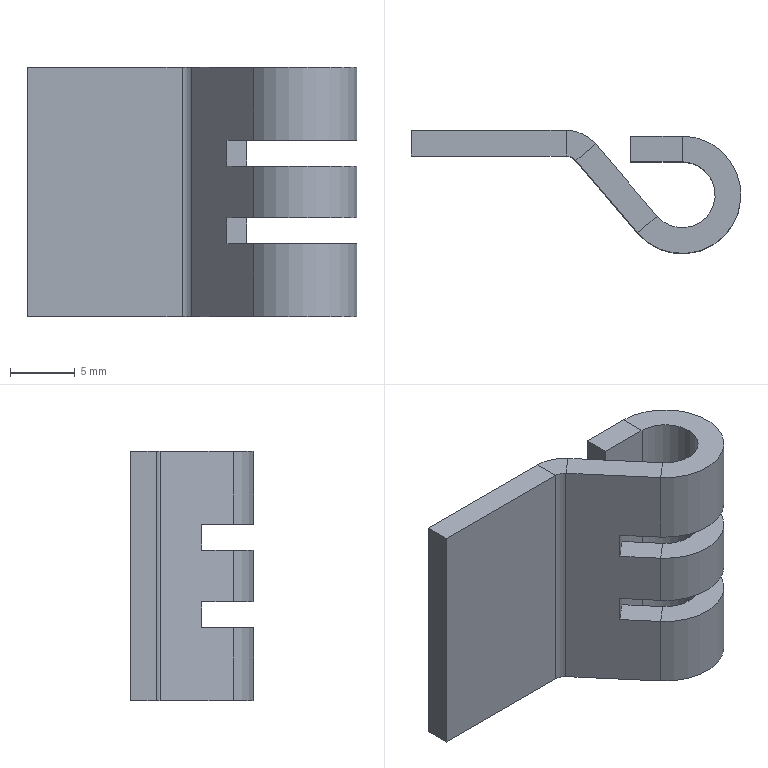Part | SolidWorks | features BaseBody 1 | 1 solid | 46 faces | box 25.55 x 9.55 x 19.3 mm | volume 1346 mm3 | plane 38 | cylinder 8 | commonest cylinder face diameters 5.1 x3 9.1 x3 2 x1 6 x1
STEP:
#1=CARTESIAN_POINT('',(15.,-2.45,-4.));
#2=VERTEX_POINT('',#1);
#3=CARTESIAN_POINT('',(15.,-0.45,-4.));
#4=VERTEX_POINT('',#3);
#5=CARTESIAN_POINT('',(15.,-2.45,-4.));
#6=DIRECTION('',(0.,1.,0.));
#7=VECTOR('',#6,1000.);
#8=LINE('',#5,#7);
#9=EDGE_CURVE('',#2,#4,#8,.T.);
#10=ORIENTED_EDGE('',*,*,#9,.F.);
#11=CARTESIAN_POINT('',(13.06,-6.655,-4.));
#12=VERTEX_POINT('',#11);
#13=CARTESIAN_POINT('',(15.,-5.,-4.));
#14=DIRECTION('',(0.,0.,1.));
#15=DIRECTION('',(-1.,0.,0.));
#16=AXIS2_PLACEMENT_3D('',#13,#14,#15);
#17=CIRCLE('',#16,2.55);
#18=EDGE_CURVE('',#12,#2,#17,.T.);
#19=ORIENTED_EDGE('',*,*,#18,.F.);
#20=CARTESIAN_POINT('',(11.538,-7.953,-4.));
#21=VERTEX_POINT('',#20);
#22=CARTESIAN_POINT('',(11.538,-7.953,-4.));
#23=DIRECTION('',(0.7609,0.6489,0.));
#24=VECTOR('',#23,1000.);
#25=LINE('',#22,#24);
#26=EDGE_CURVE('',#21,#12,#25,.T.);
#27=ORIENTED_EDGE('',*,*,#26,.F.);
#28=CARTESIAN_POINT('',(15.,-5.,-4.));
#29=DIRECTION('',(0.,0.,1.));
#30=DIRECTION('',(-1.,0.,0.));
#31=AXIS2_PLACEMENT_3D('',#28,#29,#30);
#32=CIRCLE('',#31,4.55);
#33=EDGE_CURVE('',#21,#4,#32,.T.);
#34=ORIENTED_EDGE('',*,*,#33,.T.);
#35=EDGE_LOOP('',(#10,#19,#27,#34));
#36=FACE_OUTER_BOUND('',#35,.T.);
#37=CARTESIAN_POINT('',(15.,-5.,-4.));
#38=DIRECTION('',(0.,0.,1.));
#39=DIRECTION('',(1.,0.,0.));
#40=AXIS2_PLACEMENT_3D('',#37,#38,#39);
#41=PLANE('',#40);
#42=ADVANCED_FACE('',(#36),#41,.T.);
#43=CARTESIAN_POINT('',(11.538,-7.953,-2.));
#44=VERTEX_POINT('',#43);
#45=CARTESIAN_POINT('',(13.06,-6.655,-2.));
#46=VERTEX_POINT('',#45);
#47=CARTESIAN_POINT('',(11.538,-7.953,-2.));
#48=DIRECTION('',(0.7609,0.6489,0.));
#49=VECTOR('',#48,1000.);
#50=LINE('',#47,#49);
#51=EDGE_CURVE('',#44,#46,#50,.T.);
#52=ORIENTED_EDGE('',*,*,#51,.T.);
#53=CARTESIAN_POINT('',(15.,-2.45,-2.));
#54=VERTEX_POINT('',#53);
#55=CARTESIAN_POINT('',(15.,-5.,-2.));
#56=DIRECTION('',(0.,0.,-1.));
#57=DIRECTION('',(1.,0.,0.));
#58=AXIS2_PLACEMENT_3D('',#55,#56,#57);
#59=CIRCLE('',#58,2.55);
#60=EDGE_CURVE('',#54,#46,#59,.T.);
#61=ORIENTED_EDGE('',*,*,#60,.F.);
#62=CARTESIAN_POINT('',(15.,-0.45,-2.));
#63=VERTEX_POINT('',#62);
#64=CARTESIAN_POINT('',(15.,-2.45,-2.));
#65=DIRECTION('',(0.,1.,0.));
#66=VECTOR('',#65,1000.);
#67=LINE('',#64,#66);
#68=EDGE_CURVE('',#54,#63,#67,.T.);
#69=ORIENTED_EDGE('',*,*,#68,.T.);
#70=CARTESIAN_POINT('',(15.,-5.,-2.));
#71=DIRECTION('',(0.,0.,-1.));
#72=DIRECTION('',(-1.,0.,0.));
#73=AXIS2_PLACEMENT_3D('',#70,#71,#72);
#74=CIRCLE('',#73,4.55);
#75=EDGE_CURVE('',#63,#44,#74,.T.);
#76=ORIENTED_EDGE('',*,*,#75,.T.);
#77=EDGE_LOOP('',(#52,#61,#69,#76));
#78=FACE_OUTER_BOUND('',#77,.T.);
#79=CARTESIAN_POINT('',(15.,-5.,-2.));
#80=DIRECTION('',(0.,0.,-1.));
#81=DIRECTION('',(0.,-1.,0.));
#82=AXIS2_PLACEMENT_3D('',#79,#80,#81);
#83=PLANE('',#82);
#84=ADVANCED_FACE('',(#78),#83,.T.);
#85=CARTESIAN_POINT('',(11.,-2.45,-4.));
#86=VERTEX_POINT('',#85);
#87=CARTESIAN_POINT('',(11.,-0.45,-4.));
#88=VERTEX_POINT('',#87);
#89=CARTESIAN_POINT('',(11.,-2.45,-4.));
#90=DIRECTION('',(0.,1.,0.));
#91=VECTOR('',#90,1000.);
#92=LINE('',#89,#91);
#93=EDGE_CURVE('',#86,#88,#92,.T.);
#94=ORIENTED_EDGE('',*,*,#93,.F.);
#95=CARTESIAN_POINT('',(15.,-2.45,-4.));
#96=DIRECTION('',(-1.,0.,0.));
#97=VECTOR('',#96,1000.);
#98=LINE('',#95,#97);
#99=EDGE_CURVE('',#2,#86,#98,.T.);
#100=ORIENTED_EDGE('',*,*,#99,.F.);
#101=ORIENTED_EDGE('',*,*,#9,.T.);
#102=CARTESIAN_POINT('',(15.,-0.45,-4.));
#103=DIRECTION('',(-1.,0.,0.));
#104=VECTOR('',#103,1000.);
#105=LINE('',#102,#104);
#106=EDGE_CURVE('',#4,#88,#105,.T.);
#107=ORIENTED_EDGE('',*,*,#106,.T.);
#108=EDGE_LOOP('',(#94,#100,#101,#107));
#109=FACE_OUTER_BOUND('',#108,.T.);
#110=CARTESIAN_POINT('',(15.,-2.45,-4.));
#111=DIRECTION('',(0.,0.,-1.));
#112=DIRECTION('',(0.,-1.,0.));
#113=AXIS2_PLACEMENT_3D('',#110,#111,#112);
#114=PLANE('',#113);
#115=ADVANCED_FACE('',(#109),#114,.F.);
#116=ORIENTED_EDGE('',*,*,#68,.F.);
#117=CARTESIAN_POINT('',(11.,-2.45,-2.));
#118=VERTEX_POINT('',#117);
#119=CARTESIAN_POINT('',(15.,-2.45,-2.));
#120=DIRECTION('',(1.,0.,0.));
#121=VECTOR('',#120,1000.);
#122=LINE('',#119,#121);
#123=EDGE_CURVE('',#118,#54,#122,.T.);
#124=ORIENTED_EDGE('',*,*,#123,.F.);
#125=CARTESIAN_POINT('',(11.,-0.45,-2.));
#126=VERTEX_POINT('',#125);
#127=CARTESIAN_POINT('',(11.,-2.45,-2.));
#128=DIRECTION('',(0.,1.,0.));
#129=VECTOR('',#128,1000.);
#130=LINE('',#127,#129);
#131=EDGE_CURVE('',#118,#126,#130,.T.);
#132=ORIENTED_EDGE('',*,*,#131,.T.);
#133=CARTESIAN_POINT('',(15.,-0.45,-2.));
#134=DIRECTION('',(1.,0.,0.));
#135=VECTOR('',#134,1000.);
#136=LINE('',#133,#135);
#137=EDGE_CURVE('',#126,#63,#136,.T.);
#138=ORIENTED_EDGE('',*,*,#137,.T.);
#139=EDGE_LOOP('',(#116,#124,#132,#138));
#140=FACE_OUTER_BOUND('',#139,.T.);
#141=CARTESIAN_POINT('',(15.,-2.45,-2.));
#142=DIRECTION('',(0.,0.,1.));
#143=DIRECTION('',(1.,0.,0.));
#144=AXIS2_PLACEMENT_3D('',#141,#142,#143);
#145=PLANE('',#144);
#146=ADVANCED_FACE('',(#140),#145,.F.);
#147=CARTESIAN_POINT('',(11.,-4.24,-2.));
#148=VERTEX_POINT('',#147);
#149=CARTESIAN_POINT('',(11.,-4.24,-4.));
#150=VERTEX_POINT('',#149);
#151=CARTESIAN_POINT('',(11.,-4.24,9.65));
#152=DIRECTION('',(0.,0.,-1.));
#153=VECTOR('',#152,1000.);
#154=LINE('',#151,#153);
#155=EDGE_CURVE('',#148,#150,#154,.T.);
#156=ORIENTED_EDGE('',*,*,#155,.F.);
#157=CARTESIAN_POINT('',(9.478,-5.537,-2.));
#158=VERTEX_POINT('',#157);
#159=CARTESIAN_POINT('',(11.,-4.24,-2.));
#160=DIRECTION('',(-0.7609,-0.6489,0.));
#161=VECTOR('',#160,1000.);
#162=LINE('',#159,#161);
#163=EDGE_CURVE('',#148,#158,#162,.T.);
#164=ORIENTED_EDGE('',*,*,#163,.T.);
#165=CARTESIAN_POINT('',(9.478,-5.537,-4.));
#166=VERTEX_POINT('',#165);
#167=CARTESIAN_POINT('',(9.478,-5.537,9.65));
#168=DIRECTION('',(0.,0.,-1.));
#169=VECTOR('',#168,1000.);
#170=LINE('',#167,#169);
#171=EDGE_CURVE('',#158,#166,#170,.T.);
#172=ORIENTED_EDGE('',*,*,#171,.T.);
#173=CARTESIAN_POINT('',(11.,-4.24,-4.));
#174=DIRECTION('',(-0.7609,-0.6489,0.));
#175=VECTOR('',#174,1000.);
#176=LINE('',#173,#175);
#177=EDGE_CURVE('',#150,#166,#176,.T.);
#178=ORIENTED_EDGE('',*,*,#177,.F.);
#179=EDGE_LOOP('',(#156,#164,#172,#178));
#180=FACE_OUTER_BOUND('',#179,.T.);
#181=CARTESIAN_POINT('',(11.,-4.24,9.65));
#182=DIRECTION('',(-0.6489,0.7609,0.));
#183=DIRECTION('',(0.,0.,1.));
#184=AXIS2_PLACEMENT_3D('',#181,#182,#183);
#185=PLANE('',#184);
#186=ADVANCED_FACE('',(#180),#185,.F.);
#187=CARTESIAN_POINT('',(11.538,-7.953,-4.));
#188=DIRECTION('',(0.6489,-0.7609,0.));
#189=VECTOR('',#188,1000.);
#190=LINE('',#187,#189);
#191=EDGE_CURVE('',#166,#21,#190,.T.);
#192=ORIENTED_EDGE('',*,*,#191,.T.);
#193=ORIENTED_EDGE('',*,*,#26,.T.);
#194=CARTESIAN_POINT('',(13.06,-6.655,-4.));
#195=DIRECTION('',(0.6489,-0.7609,0.));
#196=VECTOR('',#195,1000.);
#197=LINE('',#194,#196);
#198=EDGE_CURVE('',#150,#12,#197,.T.);
#199=ORIENTED_EDGE('',*,*,#198,.F.);
#200=ORIENTED_EDGE('',*,*,#177,.T.);
#201=EDGE_LOOP('',(#192,#193,#199,#200));
#202=FACE_OUTER_BOUND('',#201,.T.);
#203=CARTESIAN_POINT('',(11.538,-7.953,-4.));
#204=DIRECTION('',(0.,0.,-1.));
#205=DIRECTION('',(0.,-1.,0.));
#206=AXIS2_PLACEMENT_3D('',#203,#204,#205);
#207=PLANE('',#206);
#208=ADVANCED_FACE('',(#202),#207,.F.);
#209=ORIENTED_EDGE('',*,*,#51,.F.);
#210=CARTESIAN_POINT('',(11.538,-7.953,-2.));
#211=DIRECTION('',(-0.6489,0.7609,0.));
#212=VECTOR('',#211,1000.);
#213=LINE('',#210,#212);
#214=EDGE_CURVE('',#44,#158,#213,.T.);
#215=ORIENTED_EDGE('',*,*,#214,.T.);
#216=ORIENTED_EDGE('',*,*,#163,.F.);
#217=CARTESIAN_POINT('',(13.06,-6.655,-2.));
#218=DIRECTION('',(-0.6489,0.7609,0.));
#219=VECTOR('',#218,1000.);
#220=LINE('',#217,#219);
#221=EDGE_CURVE('',#46,#148,#220,.T.);
#222=ORIENTED_EDGE('',*,*,#221,.F.);
#223=EDGE_LOOP('',(#209,#215,#216,#222));
#224=FACE_OUTER_BOUND('',#223,.T.);
#225=CARTESIAN_POINT('',(11.538,-7.953,-2.));
#226=DIRECTION('',(0.,0.,1.));
#227=DIRECTION('',(0.,-1.,0.));
#228=AXIS2_PLACEMENT_3D('',#225,#226,#227);
#229=PLANE('',#228);
#230=ADVANCED_FACE('',(#224),#229,.F.);
#231=CARTESIAN_POINT('',(11.538,-7.953,4.));
#232=VERTEX_POINT('',#231);
#233=CARTESIAN_POINT('',(13.06,-6.655,4.));
#234=VERTEX_POINT('',#233);
#235=CARTESIAN_POINT('',(11.538,-7.953,4.));
#236=DIRECTION('',(0.7609,0.6489,0.));
#237=VECTOR('',#236,1000.);
#238=LINE('',#235,#237);
#239=EDGE_CURVE('',#232,#234,#238,.T.);
#240=ORIENTED_EDGE('',*,*,#239,.T.);
#241=CARTESIAN_POINT('',(15.,-2.45,4.));
#242=VERTEX_POINT('',#241);
#243=CARTESIAN_POINT('',(15.,-5.,4.));
#244=DIRECTION('',(0.,0.,-1.));
#245=DIRECTION('',(1.,0.,0.));
#246=AXIS2_PLACEMENT_3D('',#243,#244,#245);
#247=CIRCLE('',#246,2.55);
#248=EDGE_CURVE('',#242,#234,#247,.T.);
#249=ORIENTED_EDGE('',*,*,#248,.F.);
#250=CARTESIAN_POINT('',(15.,-0.45,4.));
#251=VERTEX_POINT('',#250);
#252=CARTESIAN_POINT('',(15.,-2.45,4.));
#253=DIRECTION('',(0.,1.,0.));
#254=VECTOR('',#253,1000.);
#255=LINE('',#252,#254);
#256=EDGE_CURVE('',#242,#251,#255,.T.);
#257=ORIENTED_EDGE('',*,*,#256,.T.);
#258=CARTESIAN_POINT('',(15.,-5.,4.));
#259=DIRECTION('',(0.,0.,-1.));
#260=DIRECTION('',(-1.,0.,0.));
#261=AXIS2_PLACEMENT_3D('',#258,#259,#260);
#262=CIRCLE('',#261,4.55);
#263=EDGE_CURVE('',#251,#232,#262,.T.);
#264=ORIENTED_EDGE('',*,*,#263,.T.);
#265=EDGE_LOOP('',(#240,#249,#257,#264));
#266=FACE_OUTER_BOUND('',#265,.T.);
#267=CARTESIAN_POINT('',(15.,-5.,4.));
#268=DIRECTION('',(0.,0.,-1.));
#269=DIRECTION('',(0.,-1.,0.));
#270=AXIS2_PLACEMENT_3D('',#267,#268,#269);
#271=PLANE('',#270);
#272=ADVANCED_FACE('',(#266),#271,.T.);
#273=CARTESIAN_POINT('',(15.,-2.45,2.));
#274=VERTEX_POINT('',#273);
#275=CARTESIAN_POINT('',(15.,-0.45,2.));
#276=VERTEX_POINT('',#275);
#277=CARTESIAN_POINT('',(15.,-2.45,2.));
#278=DIRECTION('',(0.,1.,0.));
#279=VECTOR('',#278,1000.);
#280=LINE('',#277,#279);
#281=EDGE_CURVE('',#274,#276,#280,.T.);
#282=ORIENTED_EDGE('',*,*,#281,.F.);
#283=CARTESIAN_POINT('',(13.06,-6.655,2.));
#284=VERTEX_POINT('',#283);
#285=CARTESIAN_POINT('',(15.,-5.,2.));
#286=DIRECTION('',(0.,0.,1.));
#287=DIRECTION('',(-1.,0.,0.));
#288=AXIS2_PLACEMENT_3D('',#285,#286,#287);
#289=CIRCLE('',#288,2.55);
#290=EDGE_CURVE('',#284,#274,#289,.T.);
#291=ORIENTED_EDGE('',*,*,#290,.F.);
#292=CARTESIAN_POINT('',(11.538,-7.953,2.));
#293=VERTEX_POINT('',#292);
#294=CARTESIAN_POINT('',(11.538,-7.953,2.));
#295=DIRECTION('',(0.7609,0.6489,0.));
#296=VECTOR('',#295,1000.);
#297=LINE('',#294,#296);
#298=EDGE_CURVE('',#293,#284,#297,.T.);
#299=ORIENTED_EDGE('',*,*,#298,.F.);
#300=CARTESIAN_POINT('',(15.,-5.,2.));
#301=DIRECTION('',(0.,0.,1.));
#302=DIRECTION('',(-1.,0.,0.));
#303=AXIS2_PLACEMENT_3D('',#300,#301,#302);
#304=CIRCLE('',#303,4.55);
#305=EDGE_CURVE('',#293,#276,#304,.T.);
#306=ORIENTED_EDGE('',*,*,#305,.T.);
#307=EDGE_LOOP('',(#282,#291,#299,#306));
#308=FACE_OUTER_BOUND('',#307,.T.);
#309=CARTESIAN_POINT('',(15.,-5.,2.));
#310=DIRECTION('',(0.,0.,1.));
#311=DIRECTION('',(1.,0.,0.));
#312=AXIS2_PLACEMENT_3D('',#309,#310,#311);
#313=PLANE('',#312);
#314=ADVANCED_FACE('',(#308),#313,.T.);
#315=ORIENTED_EDGE('',*,*,#256,.F.);
#316=CARTESIAN_POINT('',(11.,-2.45,4.));
#317=VERTEX_POINT('',#316);
#318=CARTESIAN_POINT('',(15.,-2.45,4.));
#319=DIRECTION('',(1.,0.,0.));
#320=VECTOR('',#319,1000.);
#321=LINE('',#318,#320);
#322=EDGE_CURVE('',#317,#242,#321,.T.);
#323=ORIENTED_EDGE('',*,*,#322,.F.);
#324=CARTESIAN_POINT('',(11.,-0.45,4.));
#325=VERTEX_POINT('',#324);
#326=CARTESIAN_POINT('',(11.,-2.45,4.));
#327=DIRECTION('',(0.,1.,0.));
#328=VECTOR('',#327,1000.);
#329=LINE('',#326,#328);
#330=EDGE_CURVE('',#317,#325,#329,.T.);
#331=ORIENTED_EDGE('',*,*,#330,.T.);
#332=CARTESIAN_POINT('',(15.,-0.45,4.));
#333=DIRECTION('',(1.,0.,0.));
#334=VECTOR('',#333,1000.);
#335=LINE('',#332,#334);
#336=EDGE_CURVE('',#325,#251,#335,.T.);
#337=ORIENTED_EDGE('',*,*,#336,.T.);
#338=EDGE_LOOP('',(#315,#323,#331,#337));
#339=FACE_OUTER_BOUND('',#338,.T.);
#340=CARTESIAN_POINT('',(15.,-2.45,4.));
#341=DIRECTION('',(0.,0.,1.));
#342=DIRECTION('',(1.,0.,0.));
#343=AXIS2_PLACEMENT_3D('',#340,#341,#342);
#344=PLANE('',#343);
#345=ADVANCED_FACE('',(#339),#344,.F.);
#346=CARTESIAN_POINT('',(11.,-2.45,2.));
#347=VERTEX_POINT('',#346);
#348=CARTESIAN_POINT('',(11.,-0.45,2.));
#349=VERTEX_POINT('',#348);
#350=CARTESIAN_POINT('',(11.,-2.45,2.));
#351=DIRECTION('',(0.,1.,0.));
#352=VECTOR('',#351,1000.);
#353=LINE('',#350,#352);
#354=EDGE_CURVE('',#347,#349,#353,.T.);
#355=ORIENTED_EDGE('',*,*,#354,.F.);
#356=CARTESIAN_POINT('',(15.,-2.45,2.));
#357=DIRECTION('',(-1.,0.,0.));
#358=VECTOR('',#357,1000.);
#359=LINE('',#356,#358);
#360=EDGE_CURVE('',#274,#347,#359,.T.);
#361=ORIENTED_EDGE('',*,*,#360,.F.);
#362=ORIENTED_EDGE('',*,*,#281,.T.);
#363=CARTESIAN_POINT('',(15.,-0.45,2.));
#364=DIRECTION('',(-1.,0.,0.));
#365=VECTOR('',#364,1000.);
#366=LINE('',#363,#365);
#367=EDGE_CURVE('',#276,#349,#366,.T.);
#368=ORIENTED_EDGE('',*,*,#367,.T.);
#369=EDGE_LOOP('',(#355,#361,#362,#368));
#370=FACE_OUTER_BOUND('',#369,.T.);
#371=CARTESIAN_POINT('',(15.,-2.45,2.));
#372=DIRECTION('',(0.,0.,-1.));
#373=DIRECTION('',(-1.,0.,0.));
#374=AXIS2_PLACEMENT_3D('',#371,#372,#373);
#375=PLANE('',#374);
#376=ADVANCED_FACE('',(#370),#375,.F.);
#377=CARTESIAN_POINT('',(11.,-4.24,2.));
#378=VERTEX_POINT('',#377);
#379=CARTESIAN_POINT('',(9.478,-5.537,2.));
#380=VERTEX_POINT('',#379);
#381=CARTESIAN_POINT('',(11.,-4.24,2.));
#382=DIRECTION('',(-0.7609,-0.6489,0.));
#383=VECTOR('',#382,1000.);
#384=LINE('',#381,#383);
#385=EDGE_CURVE('',#378,#380,#384,.T.);
#386=ORIENTED_EDGE('',*,*,#385,.F.);
#387=CARTESIAN_POINT('',(11.,-4.24,4.));
#388=VERTEX_POINT('',#387);
#389=CARTESIAN_POINT('',(11.,-4.24,9.65));
#390=DIRECTION('',(0.,0.,-1.));
#391=VECTOR('',#390,1000.);
#392=LINE('',#389,#391);
#393=EDGE_CURVE('',#388,#378,#392,.T.);
#394=ORIENTED_EDGE('',*,*,#393,.F.);
#395=CARTESIAN_POINT('',(9.478,-5.537,4.));
#396=VERTEX_POINT('',#395);
#397=CARTESIAN_POINT('',(11.,-4.24,4.));
#398=DIRECTION('',(-0.7609,-0.6489,0.));
#399=VECTOR('',#398,1000.);
#400=LINE('',#397,#399);
#401=EDGE_CURVE('',#388,#396,#400,.T.);
#402=ORIENTED_EDGE('',*,*,#401,.T.);
#403=CARTESIAN_POINT('',(9.478,-5.537,9.65));
#404=DIRECTION('',(0.,0.,-1.));
#405=VECTOR('',#404,1000.);
#406=LINE('',#403,#405);
#407=EDGE_CURVE('',#396,#380,#406,.T.);
#408=ORIENTED_EDGE('',*,*,#407,.T.);
#409=EDGE_LOOP('',(#386,#394,#402,#408));
#410=FACE_OUTER_BOUND('',#409,.T.);
#411=CARTESIAN_POINT('',(11.,-4.24,9.65));
#412=DIRECTION('',(-0.6489,0.7609,0.));
#413=DIRECTION('',(0.,0.,1.));
#414=AXIS2_PLACEMENT_3D('',#411,#412,#413);
#415=PLANE('',#414);
#416=ADVANCED_FACE('',(#410),#415,.F.);
#417=CARTESIAN_POINT('',(11.538,-7.953,4.));
#418=DIRECTION('',(-0.6489,0.7609,0.));
#419=VECTOR('',#418,1000.);
#420=LINE('',#417,#419);
#421=EDGE_CURVE('',#232,#396,#420,.T.);
#422=ORIENTED_EDGE('',*,*,#421,.T.);
#423=ORIENTED_EDGE('',*,*,#401,.F.);
#424=CARTESIAN_POINT('',(13.06,-6.655,4.));
#425=DIRECTION('',(-0.6489,0.7609,0.));
#426=VECTOR('',#425,1000.);
#427=LINE('',#424,#426);
#428=EDGE_CURVE('',#234,#388,#427,.T.);
#429=ORIENTED_EDGE('',*,*,#428,.F.);
#430=ORIENTED_EDGE('',*,*,#239,.F.);
#431=EDGE_LOOP('',(#422,#423,#429,#430));
#432=FACE_OUTER_BOUND('',#431,.T.);
#433=CARTESIAN_POINT('',(11.538,-7.953,4.));
#434=DIRECTION('',(0.,0.,1.));
#435=DIRECTION('',(1.,0.,0.));
#436=AXIS2_PLACEMENT_3D('',#433,#434,#435);
#437=PLANE('',#436);
#438=ADVANCED_FACE('',(#432),#437,.F.);
#439=CARTESIAN_POINT('',(11.538,-7.953,2.));
#440=DIRECTION('',(0.6489,-0.7609,0.));
#441=VECTOR('',#440,1000.);
#442=LINE('',#439,#441);
#443=EDGE_CURVE('',#380,#293,#442,.T.);
#444=ORIENTED_EDGE('',*,*,#443,.T.);
#445=ORIENTED_EDGE('',*,*,#298,.T.);
#446=CARTESIAN_POINT('',(13.06,-6.655,2.));
#447=DIRECTION('',(0.6489,-0.7609,0.));
#448=VECTOR('',#447,1000.);
#449=LINE('',#446,#448);
#450=EDGE_CURVE('',#378,#284,#449,.T.);
#451=ORIENTED_EDGE('',*,*,#450,.F.);
#452=ORIENTED_EDGE('',*,*,#385,.T.);
#453=EDGE_LOOP('',(#444,#445,#451,#452));
#454=FACE_OUTER_BOUND('',#453,.T.);
#455=CARTESIAN_POINT('',(11.538,-7.953,2.));
#456=DIRECTION('',(0.,0.,-1.));
#457=DIRECTION('',(-1.,0.,0.));
#458=AXIS2_PLACEMENT_3D('',#455,#456,#457);
#459=PLANE('',#458);
#460=ADVANCED_FACE('',(#454),#459,.F.);
#461=CARTESIAN_POINT('',(11.,-0.45,-9.65));
#462=VERTEX_POINT('',#461);
#463=CARTESIAN_POINT('',(15.,-0.45,-9.65));
#464=VERTEX_POINT('',#463);
#465=CARTESIAN_POINT('',(15.,-0.45,-9.65));
#466=DIRECTION('',(1.,0.,0.));
#467=VECTOR('',#466,1000.);
#468=LINE('',#465,#467);
#469=EDGE_CURVE('',#462,#464,#468,.T.);
#470=ORIENTED_EDGE('',*,*,#469,.T.);
#471=CARTESIAN_POINT('',(15.,-2.45,-9.65));
#472=VERTEX_POINT('',#471);
#473=CARTESIAN_POINT('',(15.,-0.45,-9.65));
#474=DIRECTION('',(0.,-1.,0.));
#475=VECTOR('',#474,1000.);
#476=LINE('',#473,#475);
#477=EDGE_CURVE('',#464,#472,#476,.T.);
#478=ORIENTED_EDGE('',*,*,#477,.T.);
#479=CARTESIAN_POINT('',(11.,-2.45,-9.65));
#480=VERTEX_POINT('',#479);
#481=CARTESIAN_POINT('',(15.,-2.45,-9.65));
#482=DIRECTION('',(1.,0.,0.));
#483=VECTOR('',#482,1000.);
#484=LINE('',#481,#483);
#485=EDGE_CURVE('',#480,#472,#484,.T.);
#486=ORIENTED_EDGE('',*,*,#485,.F.);
#487=CARTESIAN_POINT('',(11.,-2.45,-9.65));
#488=DIRECTION('',(0.,1.,0.));
#489=VECTOR('',#488,1000.);
#490=LINE('',#487,#489);
#491=EDGE_CURVE('',#480,#462,#490,.T.);
#492=ORIENTED_EDGE('',*,*,#491,.T.);
#493=EDGE_LOOP('',(#470,#478,#486,#492));
#494=FACE_OUTER_BOUND('',#493,.T.);
#495=CARTESIAN_POINT('',(6.,-3.,-9.65));
#496=DIRECTION('',(0.,0.,1.));
#497=DIRECTION('',(1.,0.,0.));
#498=AXIS2_PLACEMENT_3D('',#495,#496,#497);
#499=PLANE('',#498);
#500=ADVANCED_FACE('',(#494),#499,.F.);
#501=CARTESIAN_POINT('',(6.,0.,9.65));
#502=VERTEX_POINT('',#501);
#503=CARTESIAN_POINT('',(-6.,0.,9.65));
#504=VERTEX_POINT('',#503);
#505=CARTESIAN_POINT('',(6.,0.,9.65));
#506=DIRECTION('',(-1.,0.,0.));
#507=VECTOR('',#506,1000.);
#508=LINE('',#505,#507);
#509=EDGE_CURVE('',#502,#504,#508,.T.);
#510=ORIENTED_EDGE('',*,*,#509,.T.);
#511=CARTESIAN_POINT('',(-6.,-2.,9.65));
#512=VERTEX_POINT('',#511);
#513=CARTESIAN_POINT('',(-6.,-2.,9.65));
#514=DIRECTION('',(0.,1.,0.));
#515=VECTOR('',#514,1000.);
#516=LINE('',#513,#515);
#517=EDGE_CURVE('',#512,#504,#516,.T.);
#518=ORIENTED_EDGE('',*,*,#517,.F.);
#519=CARTESIAN_POINT('',(6.,-2.,9.65));
#520=VERTEX_POINT('',#519);
#521=CARTESIAN_POINT('',(6.,-2.,9.65));
#522=DIRECTION('',(-1.,0.,0.));
#523=VECTOR('',#522,1000.);
#524=LINE('',#521,#523);
#525=EDGE_CURVE('',#520,#512,#524,.T.);
#526=ORIENTED_EDGE('',*,*,#525,.F.);
#527=CARTESIAN_POINT('',(6.,-2.,9.65));
#528=DIRECTION('',(0.,1.,0.));
#529=VECTOR('',#528,1000.);
#530=LINE('',#527,#529);
#531=EDGE_CURVE('',#520,#502,#530,.T.);
#532=ORIENTED_EDGE('',*,*,#531,.T.);
#533=EDGE_LOOP('',(#510,#518,#526,#532));
#534=FACE_OUTER_BOUND('',#533,.T.);
#535=CARTESIAN_POINT('',(6.,-3.,9.65));
#536=DIRECTION('',(0.,0.,1.));
#537=DIRECTION('',(1.,0.,0.));
#538=AXIS2_PLACEMENT_3D('',#535,#536,#537);
#539=PLANE('',#538);
#540=ADVANCED_FACE('',(#534),#539,.T.);
#541=CARTESIAN_POINT('',(8.283,-1.053,-9.65));
#542=VERTEX_POINT('',#541);
#543=CARTESIAN_POINT('',(6.,0.,-9.65));
#544=VERTEX_POINT('',#543);
#545=CARTESIAN_POINT('',(6.,-3.,-9.65));
#546=DIRECTION('',(0.,0.,1.));
#547=DIRECTION('',(1.,0.,0.));
#548=AXIS2_PLACEMENT_3D('',#545,#546,#547);
#549=CIRCLE('',#548,3.);
#550=EDGE_CURVE('',#542,#544,#549,.T.);
#551=ORIENTED_EDGE('',*,*,#550,.T.);
#552=CARTESIAN_POINT('',(6.,0.,9.65));
#553=DIRECTION('',(0.,0.,-1.));
#554=VECTOR('',#553,1000.);
#555=LINE('',#552,#554);
#556=EDGE_CURVE('',#502,#544,#555,.T.);
#557=ORIENTED_EDGE('',*,*,#556,.F.);
#558=CARTESIAN_POINT('',(8.283,-1.053,9.65));
#559=VERTEX_POINT('',#558);
#560=CARTESIAN_POINT('',(6.,-3.,9.65));
#561=DIRECTION('',(0.,0.,1.));
#562=DIRECTION('',(1.,0.,0.));
#563=AXIS2_PLACEMENT_3D('',#560,#561,#562);
#564=CIRCLE('',#563,3.);
#565=EDGE_CURVE('',#559,#502,#564,.T.);
#566=ORIENTED_EDGE('',*,*,#565,.F.);
#567=CARTESIAN_POINT('',(8.283,-1.053,9.65));
#568=DIRECTION('',(0.,0.,-1.));
#569=VECTOR('',#568,1000.);
#570=LINE('',#567,#569);
#571=EDGE_CURVE('',#559,#542,#570,.T.);
#572=ORIENTED_EDGE('',*,*,#571,.T.);
#573=EDGE_LOOP('',(#551,#557,#566,#572));
#574=FACE_OUTER_BOUND('',#573,.T.);
#575=CARTESIAN_POINT('',(6.,-3.,9.65));
#576=DIRECTION('',(0.,0.,-1.));
#577=DIRECTION('',(-1.,0.,0.));
#578=AXIS2_PLACEMENT_3D('',#575,#576,#577);
#579=CYLINDRICAL_SURFACE('',#578,3.);
#580=ADVANCED_FACE('',(#574),#579,.T.);
#581=CARTESIAN_POINT('',(6.761,-2.351,-9.65));
#582=VERTEX_POINT('',#581);
#583=CARTESIAN_POINT('',(6.,-2.,-9.65));
#584=VERTEX_POINT('',#583);
#585=CARTESIAN_POINT('',(6.,-3.,-9.65));
#586=DIRECTION('',(0.,0.,1.));
#587=DIRECTION('',(1.,0.,0.));
#588=AXIS2_PLACEMENT_3D('',#585,#586,#587);
#589=CIRCLE('',#588,1.);
#590=EDGE_CURVE('',#582,#584,#589,.T.);
#591=ORIENTED_EDGE('',*,*,#590,.F.);
#592=CARTESIAN_POINT('',(6.761,-2.351,9.65));
#593=VERTEX_POINT('',#592);
#594=CARTESIAN_POINT('',(6.761,-2.351,9.65));
#595=DIRECTION('',(0.,0.,-1.));
#596=VECTOR('',#595,1000.);
#597=LINE('',#594,#596);
#598=EDGE_CURVE('',#593,#582,#597,.T.);
#599=ORIENTED_EDGE('',*,*,#598,.F.);
#600=CARTESIAN_POINT('',(6.,-3.,9.65));
#601=DIRECTION('',(0.,0.,1.));
#602=DIRECTION('',(1.,0.,0.));
#603=AXIS2_PLACEMENT_3D('',#600,#601,#602);
#604=CIRCLE('',#603,1.);
#605=EDGE_CURVE('',#593,#520,#604,.T.);
#606=ORIENTED_EDGE('',*,*,#605,.T.);
#607=CARTESIAN_POINT('',(6.,-2.,9.65));
#608=DIRECTION('',(0.,0.,-1.));
#609=VECTOR('',#608,1000.);
#610=LINE('',#607,#609);
#611=EDGE_CURVE('',#520,#584,#610,.T.);
#612=ORIENTED_EDGE('',*,*,#611,.T.);
#613=EDGE_LOOP('',(#591,#599,#606,#612));
#614=FACE_OUTER_BOUND('',#613,.T.);
#615=CARTESIAN_POINT('',(6.,-3.,9.65));
#616=DIRECTION('',(0.,0.,-1.));
#617=DIRECTION('',(-1.,0.,0.));
#618=AXIS2_PLACEMENT_3D('',#615,#616,#617);
#619=CYLINDRICAL_SURFACE('',#618,1.);
#620=ADVANCED_FACE('',(#614),#619,.F.);
#621=ORIENTED_EDGE('',*,*,#525,.T.);
#622=CARTESIAN_POINT('',(-6.,-2.,-9.65));
#623=VERTEX_POINT('',#622);
#624=CARTESIAN_POINT('',(-6.,-2.,9.65));
#625=DIRECTION('',(0.,0.,-1.));
#626=VECTOR('',#625,1000.);
#627=LINE('',#624,#626);
#628=EDGE_CURVE('',#512,#623,#627,.T.);
#629=ORIENTED_EDGE('',*,*,#628,.T.);
#630=CARTESIAN_POINT('',(6.,-2.,-9.65));
#631=DIRECTION('',(-1.,0.,0.));
#632=VECTOR('',#631,1000.);
#633=LINE('',#630,#632);
#634=EDGE_CURVE('',#584,#623,#633,.T.);
#635=ORIENTED_EDGE('',*,*,#634,.F.);
#636=ORIENTED_EDGE('',*,*,#611,.F.);
#637=EDGE_LOOP('',(#621,#629,#635,#636));
#638=FACE_OUTER_BOUND('',#637,.T.);
#639=CARTESIAN_POINT('',(6.,-2.,9.65));
#640=DIRECTION('',(0.,-1.,0.));
#641=DIRECTION('',(0.,0.,-1.));
#642=AXIS2_PLACEMENT_3D('',#639,#640,#641);
#643=PLANE('',#642);
#644=ADVANCED_FACE('',(#638),#643,.T.);
#645=CARTESIAN_POINT('',(-6.,0.,-9.65));
#646=VERTEX_POINT('',#645);
#647=CARTESIAN_POINT('',(-6.,-2.,-9.65));
#648=DIRECTION('',(0.,1.,0.));
#649=VECTOR('',#648,1000.);
#650=LINE('',#647,#649);
#651=EDGE_CURVE('',#623,#646,#650,.T.);
#652=ORIENTED_EDGE('',*,*,#651,.F.);
#653=ORIENTED_EDGE('',*,*,#628,.F.);
#654=ORIENTED_EDGE('',*,*,#517,.T.);
#655=CARTESIAN_POINT('',(-6.,0.,9.65));
#656=DIRECTION('',(0.,0.,-1.));
#657=VECTOR('',#656,1000.);
#658=LINE('',#655,#657);
#659=EDGE_CURVE('',#504,#646,#658,.T.);
#660=ORIENTED_EDGE('',*,*,#659,.T.);
#661=EDGE_LOOP('',(#652,#653,#654,#660));
#662=FACE_OUTER_BOUND('',#661,.T.);
#663=CARTESIAN_POINT('',(-6.,-2.,9.65));
#664=DIRECTION('',(-1.,0.,0.));
#665=DIRECTION('',(0.,1.,0.));
#666=AXIS2_PLACEMENT_3D('',#663,#664,#665);
#667=PLANE('',#666);
#668=ADVANCED_FACE('',(#662),#667,.T.);
#669=CARTESIAN_POINT('',(6.,0.,-9.65));
#670=DIRECTION('',(-1.,0.,0.));
#671=VECTOR('',#670,1000.);
#672=LINE('',#669,#671);
#673=EDGE_CURVE('',#544,#646,#672,.T.);
#674=ORIENTED_EDGE('',*,*,#673,.T.);
#675=ORIENTED_EDGE('',*,*,#659,.F.);
#676=ORIENTED_EDGE('',*,*,#509,.F.);
#677=ORIENTED_EDGE('',*,*,#556,.T.);
#678=EDGE_LOOP('',(#674,#675,#676,#677));
#679=FACE_OUTER_BOUND('',#678,.T.);
#680=CARTESIAN_POINT('',(6.,0.,9.65));
#681=DIRECTION('',(0.,-1.,0.));
#682=DIRECTION('',(0.,0.,-1.));
#683=AXIS2_PLACEMENT_3D('',#680,#681,#682);
#684=PLANE('',#683);
#685=ADVANCED_FACE('',(#679),#684,.F.);
#686=ORIENTED_EDGE('',*,*,#634,.T.);
#687=ORIENTED_EDGE('',*,*,#651,.T.);
#688=ORIENTED_EDGE('',*,*,#673,.F.);
#689=CARTESIAN_POINT('',(6.,0.,-9.65));
#690=DIRECTION('',(0.,-1.,0.));
#691=VECTOR('',#690,1000.);
#692=LINE('',#689,#691);
#693=EDGE_CURVE('',#544,#584,#692,.T.);
#694=ORIENTED_EDGE('',*,*,#693,.T.);
#695=EDGE_LOOP('',(#686,#687,#688,#694));
#696=FACE_OUTER_BOUND('',#695,.T.);
#697=CARTESIAN_POINT('',(6.761,-2.351,-9.65));
#698=DIRECTION('',(0.,0.,-1.));
#699=DIRECTION('',(0.,-1.,0.));
#700=AXIS2_PLACEMENT_3D('',#697,#698,#699);
#701=PLANE('',#700);
#702=ADVANCED_FACE('',(#696),#701,.T.);
#703=ORIENTED_EDGE('',*,*,#693,.F.);
#704=ORIENTED_EDGE('',*,*,#550,.F.);
#705=CARTESIAN_POINT('',(6.761,-2.351,-9.65));
#706=DIRECTION('',(0.7609,0.6489,0.));
#707=VECTOR('',#706,1000.);
#708=LINE('',#705,#707);
#709=EDGE_CURVE('',#582,#542,#708,.T.);
#710=ORIENTED_EDGE('',*,*,#709,.F.);
#711=ORIENTED_EDGE('',*,*,#590,.T.);
#712=EDGE_LOOP('',(#703,#704,#710,#711));
#713=FACE_OUTER_BOUND('',#712,.T.);
#714=CARTESIAN_POINT('',(6.,0.,-9.65));
#715=DIRECTION('',(0.,0.,-1.));
#716=DIRECTION('',(0.,-1.,0.));
#717=AXIS2_PLACEMENT_3D('',#714,#715,#716);
#718=PLANE('',#717);
#719=ADVANCED_FACE('',(#713),#718,.T.);
#720=CARTESIAN_POINT('',(13.06,-6.655,9.65));
#721=VERTEX_POINT('',#720);
#722=CARTESIAN_POINT('',(13.06,-6.655,9.65));
#723=DIRECTION('',(-0.6489,0.7609,0.));
#724=VECTOR('',#723,1000.);
#725=LINE('',#722,#724);
#726=EDGE_CURVE('',#721,#559,#725,.T.);
#727=ORIENTED_EDGE('',*,*,#726,.T.);
#728=CARTESIAN_POINT('',(8.283,-1.053,9.65));
#729=DIRECTION('',(-0.7609,-0.6489,0.));
#730=VECTOR('',#729,1000.);
#731=LINE('',#728,#730);
#732=EDGE_CURVE('',#559,#593,#731,.T.);
#733=ORIENTED_EDGE('',*,*,#732,.T.);
#734=CARTESIAN_POINT('',(11.538,-7.953,9.65));
#735=VERTEX_POINT('',#734);
#736=CARTESIAN_POINT('',(11.538,-7.953,9.65));
#737=DIRECTION('',(-0.6489,0.7609,0.));
#738=VECTOR('',#737,1000.);
#739=LINE('',#736,#738);
#740=EDGE_CURVE('',#735,#593,#739,.T.);
#741=ORIENTED_EDGE('',*,*,#740,.F.);
#742=CARTESIAN_POINT('',(11.538,-7.953,9.65));
#743=DIRECTION('',(0.7609,0.6489,0.));
#744=VECTOR('',#743,1000.);
#745=LINE('',#742,#744);
#746=EDGE_CURVE('',#735,#721,#745,.T.);
#747=ORIENTED_EDGE('',*,*,#746,.T.);
#748=EDGE_LOOP('',(#727,#733,#741,#747));
#749=FACE_OUTER_BOUND('',#748,.T.);
#750=CARTESIAN_POINT('',(6.,-2.,9.65));
#751=DIRECTION('',(0.,0.,1.));
#752=DIRECTION('',(1.,0.,0.));
#753=AXIS2_PLACEMENT_3D('',#750,#751,#752);
#754=PLANE('',#753);
#755=ADVANCED_FACE('',(#749),#754,.T.);
#756=ORIENTED_EDGE('',*,*,#732,.F.);
#757=ORIENTED_EDGE('',*,*,#565,.T.);
#758=ORIENTED_EDGE('',*,*,#531,.F.);
#759=ORIENTED_EDGE('',*,*,#605,.F.);
#760=EDGE_LOOP('',(#756,#757,#758,#759));
#761=FACE_OUTER_BOUND('',#760,.T.);
#762=CARTESIAN_POINT('',(8.283,-1.053,9.65));
#763=DIRECTION('',(0.,0.,1.));
#764=DIRECTION('',(1.,0.,0.));
#765=AXIS2_PLACEMENT_3D('',#762,#763,#764);
#766=PLANE('',#765);
#767=ADVANCED_FACE('',(#761),#766,.T.);
#768=CARTESIAN_POINT('',(13.06,-6.655,-9.65));
#769=VERTEX_POINT('',#768);
#770=CARTESIAN_POINT('',(13.06,-6.655,-9.65));
#771=DIRECTION('',(-0.6489,0.7609,0.));
#772=VECTOR('',#771,1000.);
#773=LINE('',#770,#772);
#774=EDGE_CURVE('',#769,#542,#773,.T.);
#775=ORIENTED_EDGE('',*,*,#774,.F.);
#776=CARTESIAN_POINT('',(11.538,-7.953,-9.65));
#777=VERTEX_POINT('',#776);
#778=CARTESIAN_POINT('',(13.06,-6.655,-9.65));
#779=DIRECTION('',(-0.7609,-0.6489,0.));
#780=VECTOR('',#779,1000.);
#781=LINE('',#778,#780);
#782=EDGE_CURVE('',#769,#777,#781,.T.);
#783=ORIENTED_EDGE('',*,*,#782,.T.);
#784=CARTESIAN_POINT('',(11.538,-7.953,-9.65));
#785=DIRECTION('',(-0.6489,0.7609,0.));
#786=VECTOR('',#785,1000.);
#787=LINE('',#784,#786);
#788=EDGE_CURVE('',#777,#582,#787,.T.);
#789=ORIENTED_EDGE('',*,*,#788,.T.);
#790=ORIENTED_EDGE('',*,*,#709,.T.);
#791=EDGE_LOOP('',(#775,#783,#789,#790));
#792=FACE_OUTER_BOUND('',#791,.T.);
#793=CARTESIAN_POINT('',(15.,-0.45,-9.65));
#794=DIRECTION('',(0.,0.,-1.));
#795=DIRECTION('',(0.,-1.,0.));
#796=AXIS2_PLACEMENT_3D('',#793,#794,#795);
#797=PLANE('',#796);
#798=ADVANCED_FACE('',(#792),#797,.T.);
#799=ORIENTED_EDGE('',*,*,#782,.F.);
#800=CARTESIAN_POINT('',(15.,-5.,-9.65));
#801=DIRECTION('',(0.,0.,-1.));
#802=DIRECTION('',(1.,0.,0.));
#803=AXIS2_PLACEMENT_3D('',#800,#801,#802);
#804=CIRCLE('',#803,2.55);
#805=EDGE_CURVE('',#472,#769,#804,.T.);
#806=ORIENTED_EDGE('',*,*,#805,.F.);
#807=ORIENTED_EDGE('',*,*,#477,.F.);
#808=CARTESIAN_POINT('',(15.,-5.,-9.65));
#809=DIRECTION('',(0.,0.,-1.));
#810=DIRECTION('',(1.,0.,0.));
#811=AXIS2_PLACEMENT_3D('',#808,#809,#810);
#812=CIRCLE('',#811,4.55);
#813=EDGE_CURVE('',#464,#777,#812,.T.);
#814=ORIENTED_EDGE('',*,*,#813,.T.);
#815=EDGE_LOOP('',(#799,#806,#807,#814));
#816=FACE_OUTER_BOUND('',#815,.T.);
#817=CARTESIAN_POINT('',(13.06,-6.655,-9.65));
#818=DIRECTION('',(0.,0.,-1.));
#819=DIRECTION('',(0.,-1.,0.));
#820=AXIS2_PLACEMENT_3D('',#817,#818,#819);
#821=PLANE('',#820);
#822=ADVANCED_FACE('',(#816),#821,.T.);
#823=CARTESIAN_POINT('',(11.,-2.45,9.65));
#824=VERTEX_POINT('',#823);
#825=CARTESIAN_POINT('',(15.,-2.45,9.65));
#826=VERTEX_POINT('',#825);
#827=CARTESIAN_POINT('',(15.,-2.45,9.65));
#828=DIRECTION('',(1.,0.,0.));
#829=VECTOR('',#828,1000.);
#830=LINE('',#827,#829);
#831=EDGE_CURVE('',#824,#826,#830,.T.);
#832=ORIENTED_EDGE('',*,*,#831,.T.);
#833=CARTESIAN_POINT('',(15.,-0.45,9.65));
#834=VERTEX_POINT('',#833);
#835=CARTESIAN_POINT('',(15.,-2.45,9.65));
#836=DIRECTION('',(0.,1.,0.));
#837=VECTOR('',#836,1000.);
#838=LINE('',#835,#837);
#839=EDGE_CURVE('',#826,#834,#838,.T.);
#840=ORIENTED_EDGE('',*,*,#839,.T.);
#841=CARTESIAN_POINT('',(11.,-0.45,9.65));
#842=VERTEX_POINT('',#841);
#843=CARTESIAN_POINT('',(15.,-0.45,9.65));
#844=DIRECTION('',(1.,0.,0.));
#845=VECTOR('',#844,1000.);
#846=LINE('',#843,#845);
#847=EDGE_CURVE('',#842,#834,#846,.T.);
#848=ORIENTED_EDGE('',*,*,#847,.F.);
#849=CARTESIAN_POINT('',(11.,-2.45,9.65));
#850=DIRECTION('',(0.,1.,0.));
#851=VECTOR('',#850,1000.);
#852=LINE('',#849,#851);
#853=EDGE_CURVE('',#824,#842,#852,.T.);
#854=ORIENTED_EDGE('',*,*,#853,.F.);
#855=EDGE_LOOP('',(#832,#840,#848,#854));
#856=FACE_OUTER_BOUND('',#855,.T.);
#857=CARTESIAN_POINT('',(11.538,-7.953,9.65));
#858=DIRECTION('',(0.,0.,1.));
#859=DIRECTION('',(1.,0.,0.));
#860=AXIS2_PLACEMENT_3D('',#857,#858,#859);
#861=PLANE('',#860);
#862=ADVANCED_FACE('',(#856),#861,.T.);
#863=ORIENTED_EDGE('',*,*,#839,.F.);
#864=CARTESIAN_POINT('',(15.,-5.,9.65));
#865=DIRECTION('',(0.,0.,-1.));
#866=DIRECTION('',(1.,0.,0.));
#867=AXIS2_PLACEMENT_3D('',#864,#865,#866);
#868=CIRCLE('',#867,2.55);
#869=EDGE_CURVE('',#826,#721,#868,.T.);
#870=ORIENTED_EDGE('',*,*,#869,.T.);
#871=ORIENTED_EDGE('',*,*,#746,.F.);
#872=CARTESIAN_POINT('',(15.,-5.,9.65));
#873=DIRECTION('',(0.,0.,-1.));
#874=DIRECTION('',(1.,0.,0.));
#875=AXIS2_PLACEMENT_3D('',#872,#873,#874);
#876=CIRCLE('',#875,4.55);
#877=EDGE_CURVE('',#834,#735,#876,.T.);
#878=ORIENTED_EDGE('',*,*,#877,.F.);
#879=EDGE_LOOP('',(#863,#870,#871,#878));
#880=FACE_OUTER_BOUND('',#879,.T.);
#881=CARTESIAN_POINT('',(15.,-2.45,9.65));
#882=DIRECTION('',(0.,0.,1.));
#883=DIRECTION('',(1.,0.,0.));
#884=AXIS2_PLACEMENT_3D('',#881,#882,#883);
#885=PLANE('',#884);
#886=ADVANCED_FACE('',(#880),#885,.T.);
#887=ORIENTED_EDGE('',*,*,#248,.T.);
#888=CARTESIAN_POINT('',(13.06,-6.655,9.65));
#889=DIRECTION('',(0.,0.,-1.));
#890=VECTOR('',#889,1000.);
#891=LINE('',#888,#890);
#892=EDGE_CURVE('',#721,#234,#891,.T.);
#893=ORIENTED_EDGE('',*,*,#892,.F.);
#894=ORIENTED_EDGE('',*,*,#869,.F.);
#895=CARTESIAN_POINT('',(15.,-2.45,9.65));
#896=DIRECTION('',(0.,0.,-1.));
#897=VECTOR('',#896,1000.);
#898=LINE('',#895,#897);
#899=EDGE_CURVE('',#826,#242,#898,.T.);
#900=ORIENTED_EDGE('',*,*,#899,.T.);
#901=EDGE_LOOP('',(#887,#893,#894,#900));
#902=FACE_OUTER_BOUND('',#901,.T.);
#903=CARTESIAN_POINT('',(15.,-5.,9.65));
#904=DIRECTION('',(0.,0.,-1.));
#905=DIRECTION('',(-1.,0.,0.));
#906=AXIS2_PLACEMENT_3D('',#903,#904,#905);
#907=CYLINDRICAL_SURFACE('',#906,2.55);
#908=ADVANCED_FACE('',(#902),#907,.F.);
#909=ORIENTED_EDGE('',*,*,#322,.T.);
#910=ORIENTED_EDGE('',*,*,#899,.F.);
#911=ORIENTED_EDGE('',*,*,#831,.F.);
#912=CARTESIAN_POINT('',(11.,-2.45,9.65));
#913=DIRECTION('',(0.,0.,-1.));
#914=VECTOR('',#913,1000.);
#915=LINE('',#912,#914);
#916=EDGE_CURVE('',#824,#317,#915,.T.);
#917=ORIENTED_EDGE('',*,*,#916,.T.);
#918=EDGE_LOOP('',(#909,#910,#911,#917));
#919=FACE_OUTER_BOUND('',#918,.T.);
#920=CARTESIAN_POINT('',(15.,-2.45,9.65));
#921=DIRECTION('',(0.,1.,0.));
#922=DIRECTION('',(1.,0.,0.));
#923=AXIS2_PLACEMENT_3D('',#920,#921,#922);
#924=PLANE('',#923);
#925=ADVANCED_FACE('',(#919),#924,.F.);
#926=CARTESIAN_POINT('',(11.,-0.45,9.65));
#927=DIRECTION('',(0.,0.,-1.));
#928=VECTOR('',#927,1000.);
#929=LINE('',#926,#928);
#930=EDGE_CURVE('',#842,#325,#929,.T.);
#931=ORIENTED_EDGE('',*,*,#930,.T.);
#932=ORIENTED_EDGE('',*,*,#330,.F.);
#933=ORIENTED_EDGE('',*,*,#916,.F.);
#934=ORIENTED_EDGE('',*,*,#853,.T.);
#935=EDGE_LOOP('',(#931,#932,#933,#934));
#936=FACE_OUTER_BOUND('',#935,.T.);
#937=CARTESIAN_POINT('',(11.,-2.45,9.65));
#938=DIRECTION('',(-1.,0.,0.));
#939=DIRECTION('',(0.,0.,1.));
#940=AXIS2_PLACEMENT_3D('',#937,#938,#939);
#941=PLANE('',#940);
#942=ADVANCED_FACE('',(#936),#941,.T.);
#943=CARTESIAN_POINT('',(15.,-0.45,9.65));
#944=DIRECTION('',(0.,0.,-1.));
#945=VECTOR('',#944,1000.);
#946=LINE('',#943,#945);
#947=EDGE_CURVE('',#834,#251,#946,.T.);
#948=ORIENTED_EDGE('',*,*,#947,.T.);
#949=ORIENTED_EDGE('',*,*,#336,.F.);
#950=ORIENTED_EDGE('',*,*,#930,.F.);
#951=ORIENTED_EDGE('',*,*,#847,.T.);
#952=EDGE_LOOP('',(#948,#949,#950,#951));
#953=FACE_OUTER_BOUND('',#952,.T.);
#954=CARTESIAN_POINT('',(15.,-0.45,9.65));
#955=DIRECTION('',(0.,1.,0.));
#956=DIRECTION('',(1.,0.,0.));
#957=AXIS2_PLACEMENT_3D('',#954,#955,#956);
#958=PLANE('',#957);
#959=ADVANCED_FACE('',(#953),#958,.T.);
#960=CARTESIAN_POINT('',(11.538,-7.953,9.65));
#961=DIRECTION('',(0.,0.,-1.));
#962=VECTOR('',#961,1000.);
#963=LINE('',#960,#962);
#964=EDGE_CURVE('',#735,#232,#963,.T.);
#965=ORIENTED_EDGE('',*,*,#964,.T.);
#966=ORIENTED_EDGE('',*,*,#263,.F.);
#967=ORIENTED_EDGE('',*,*,#947,.F.);
#968=ORIENTED_EDGE('',*,*,#877,.T.);
#969=EDGE_LOOP('',(#965,#966,#967,#968));
#970=FACE_OUTER_BOUND('',#969,.T.);
#971=CARTESIAN_POINT('',(15.,-5.,9.65));
#972=DIRECTION('',(0.,0.,-1.));
#973=DIRECTION('',(-1.,0.,0.));
#974=AXIS2_PLACEMENT_3D('',#971,#972,#973);
#975=CYLINDRICAL_SURFACE('',#974,4.55);
#976=ADVANCED_FACE('',(#970),#975,.T.);
#977=ORIENTED_EDGE('',*,*,#221,.T.);
#978=ORIENTED_EDGE('',*,*,#155,.T.);
#979=ORIENTED_EDGE('',*,*,#198,.T.);
#980=CARTESIAN_POINT('',(13.06,-6.655,9.65));
#981=DIRECTION('',(0.,0.,-1.));
#982=VECTOR('',#981,1000.);
#983=LINE('',#980,#982);
#984=EDGE_CURVE('',#12,#769,#983,.T.);
#985=ORIENTED_EDGE('',*,*,#984,.T.);
#986=ORIENTED_EDGE('',*,*,#774,.T.);
#987=ORIENTED_EDGE('',*,*,#571,.F.);
#988=ORIENTED_EDGE('',*,*,#726,.F.);
#989=ORIENTED_EDGE('',*,*,#892,.T.);
#990=ORIENTED_EDGE('',*,*,#428,.T.);
#991=ORIENTED_EDGE('',*,*,#393,.T.);
#992=ORIENTED_EDGE('',*,*,#450,.T.);
#993=CARTESIAN_POINT('',(13.06,-6.655,9.65));
#994=DIRECTION('',(0.,0.,-1.));
#995=VECTOR('',#994,1000.);
#996=LINE('',#993,#995);
#997=EDGE_CURVE('',#284,#46,#996,.T.);
#998=ORIENTED_EDGE('',*,*,#997,.T.);
#999=EDGE_LOOP('',(#977,#978,#979,#985,#986,#987,#988,#989,#990,#991,#992,#998));
#1000=FACE_OUTER_BOUND('',#999,.T.);
#1001=CARTESIAN_POINT('',(13.06,-6.655,9.65));
#1002=DIRECTION('',(-0.7609,-0.6489,0.));
#1003=DIRECTION('',(-0.6489,0.7609,0.));
#1004=AXIS2_PLACEMENT_3D('',#1001,#1002,#1003);
#1005=PLANE('',#1004);
#1006=ADVANCED_FACE('',(#1000),#1005,.F.);
#1007=ORIENTED_EDGE('',*,*,#18,.T.);
#1008=CARTESIAN_POINT('',(15.,-2.45,9.65));
#1009=DIRECTION('',(0.,0.,-1.));
#1010=VECTOR('',#1009,1000.);
#1011=LINE('',#1008,#1010);
#1012=EDGE_CURVE('',#2,#472,#1011,.T.);
#1013=ORIENTED_EDGE('',*,*,#1012,.T.);
#1014=ORIENTED_EDGE('',*,*,#805,.T.);
#1015=ORIENTED_EDGE('',*,*,#984,.F.);
#1016=EDGE_LOOP('',(#1007,#1013,#1014,#1015));
#1017=FACE_OUTER_BOUND('',#1016,.T.);
#1018=CARTESIAN_POINT('',(15.,-5.,9.65));
#1019=DIRECTION('',(0.,0.,-1.));
#1020=DIRECTION('',(-1.,0.,0.));
#1021=AXIS2_PLACEMENT_3D('',#1018,#1019,#1020);
#1022=CYLINDRICAL_SURFACE('',#1021,2.55);
#1023=ADVANCED_FACE('',(#1017),#1022,.F.);
#1024=ORIENTED_EDGE('',*,*,#60,.T.);
#1025=ORIENTED_EDGE('',*,*,#997,.F.);
#1026=ORIENTED_EDGE('',*,*,#290,.T.);
#1027=CARTESIAN_POINT('',(15.,-2.45,9.65));
#1028=DIRECTION('',(0.,0.,-1.));
#1029=VECTOR('',#1028,1000.);
#1030=LINE('',#1027,#1029);
#1031=EDGE_CURVE('',#274,#54,#1030,.T.);
#1032=ORIENTED_EDGE('',*,*,#1031,.T.);
#1033=EDGE_LOOP('',(#1024,#1025,#1026,#1032));
#1034=FACE_OUTER_BOUND('',#1033,.T.);
#1035=CARTESIAN_POINT('',(15.,-5.,9.65));
#1036=DIRECTION('',(0.,0.,-1.));
#1037=DIRECTION('',(-1.,0.,0.));
#1038=AXIS2_PLACEMENT_3D('',#1035,#1036,#1037);
#1039=CYLINDRICAL_SURFACE('',#1038,2.55);
#1040=ADVANCED_FACE('',(#1034),#1039,.F.);
#1041=ORIENTED_EDGE('',*,*,#99,.T.);
#1042=CARTESIAN_POINT('',(11.,-2.45,9.65));
#1043=DIRECTION('',(0.,0.,-1.));
#1044=VECTOR('',#1043,1000.);
#1045=LINE('',#1042,#1044);
#1046=EDGE_CURVE('',#86,#480,#1045,.T.);
#1047=ORIENTED_EDGE('',*,*,#1046,.T.);
#1048=ORIENTED_EDGE('',*,*,#485,.T.);
#1049=ORIENTED_EDGE('',*,*,#1012,.F.);
#1050=EDGE_LOOP('',(#1041,#1047,#1048,#1049));
#1051=FACE_OUTER_BOUND('',#1050,.T.);
#1052=CARTESIAN_POINT('',(15.,-2.45,9.65));
#1053=DIRECTION('',(0.,1.,0.));
#1054=DIRECTION('',(1.,0.,0.));
#1055=AXIS2_PLACEMENT_3D('',#1052,#1053,#1054);
#1056=PLANE('',#1055);
#1057=ADVANCED_FACE('',(#1051),#1056,.F.);
#1058=ORIENTED_EDGE('',*,*,#123,.T.);
#1059=ORIENTED_EDGE('',*,*,#1031,.F.);
#1060=ORIENTED_EDGE('',*,*,#360,.T.);
#1061=CARTESIAN_POINT('',(11.,-2.45,9.65));
#1062=DIRECTION('',(0.,0.,-1.));
#1063=VECTOR('',#1062,1000.);
#1064=LINE('',#1061,#1063);
#1065=EDGE_CURVE('',#347,#118,#1064,.T.);
#1066=ORIENTED_EDGE('',*,*,#1065,.T.);
#1067=EDGE_LOOP('',(#1058,#1059,#1060,#1066));
#1068=FACE_OUTER_BOUND('',#1067,.T.);
#1069=CARTESIAN_POINT('',(15.,-2.45,9.65));
#1070=DIRECTION('',(0.,1.,0.));
#1071=DIRECTION('',(1.,0.,0.));
#1072=AXIS2_PLACEMENT_3D('',#1069,#1070,#1071);
#1073=PLANE('',#1072);
#1074=ADVANCED_FACE('',(#1068),#1073,.F.);
#1075=ORIENTED_EDGE('',*,*,#1046,.F.);
#1076=ORIENTED_EDGE('',*,*,#93,.T.);
#1077=CARTESIAN_POINT('',(11.,-0.45,9.65));
#1078=DIRECTION('',(0.,0.,-1.));
#1079=VECTOR('',#1078,1000.);
#1080=LINE('',#1077,#1079);
#1081=EDGE_CURVE('',#88,#462,#1080,.T.);
#1082=ORIENTED_EDGE('',*,*,#1081,.T.);
#1083=ORIENTED_EDGE('',*,*,#491,.F.);
#1084=EDGE_LOOP('',(#1075,#1076,#1082,#1083));
#1085=FACE_OUTER_BOUND('',#1084,.T.);
#1086=CARTESIAN_POINT('',(11.,-2.45,9.65));
#1087=DIRECTION('',(-1.,0.,0.));
#1088=DIRECTION('',(0.,0.,1.));
#1089=AXIS2_PLACEMENT_3D('',#1086,#1087,#1088);
#1090=PLANE('',#1089);
#1091=ADVANCED_FACE('',(#1085),#1090,.T.);
#1092=CARTESIAN_POINT('',(11.,-0.45,9.65));
#1093=DIRECTION('',(0.,0.,-1.));
#1094=VECTOR('',#1093,1000.);
#1095=LINE('',#1092,#1094);
#1096=EDGE_CURVE('',#349,#126,#1095,.T.);
#1097=ORIENTED_EDGE('',*,*,#1096,.T.);
#1098=ORIENTED_EDGE('',*,*,#131,.F.);
#1099=ORIENTED_EDGE('',*,*,#1065,.F.);
#1100=ORIENTED_EDGE('',*,*,#354,.T.);
#1101=EDGE_LOOP('',(#1097,#1098,#1099,#1100));
#1102=FACE_OUTER_BOUND('',#1101,.T.);
#1103=CARTESIAN_POINT('',(11.,-2.45,9.65));
#1104=DIRECTION('',(-1.,0.,0.));
#1105=DIRECTION('',(0.,0.,1.));
#1106=AXIS2_PLACEMENT_3D('',#1103,#1104,#1105);
#1107=PLANE('',#1106);
#1108=ADVANCED_FACE('',(#1102),#1107,.T.);
#1109=ORIENTED_EDGE('',*,*,#1081,.F.);
#1110=ORIENTED_EDGE('',*,*,#106,.F.);
#1111=CARTESIAN_POINT('',(15.,-0.45,9.65));
#1112=DIRECTION('',(0.,0.,-1.));
#1113=VECTOR('',#1112,1000.);
#1114=LINE('',#1111,#1113);
#1115=EDGE_CURVE('',#4,#464,#1114,.T.);
#1116=ORIENTED_EDGE('',*,*,#1115,.T.);
#1117=ORIENTED_EDGE('',*,*,#469,.F.);
#1118=EDGE_LOOP('',(#1109,#1110,#1116,#1117));
#1119=FACE_OUTER_BOUND('',#1118,.T.);
#1120=CARTESIAN_POINT('',(15.,-0.45,9.65));
#1121=DIRECTION('',(0.,1.,0.));
#1122=DIRECTION('',(1.,0.,0.));
#1123=AXIS2_PLACEMENT_3D('',#1120,#1121,#1122);
#1124=PLANE('',#1123);
#1125=ADVANCED_FACE('',(#1119),#1124,.T.);
#1126=CARTESIAN_POINT('',(15.,-0.45,9.65));
#1127=DIRECTION('',(0.,0.,-1.));
#1128=VECTOR('',#1127,1000.);
#1129=LINE('',#1126,#1128);
#1130=EDGE_CURVE('',#276,#63,#1129,.T.);
#1131=ORIENTED_EDGE('',*,*,#1130,.T.);
#1132=ORIENTED_EDGE('',*,*,#137,.F.);
#1133=ORIENTED_EDGE('',*,*,#1096,.F.);
#1134=ORIENTED_EDGE('',*,*,#367,.F.);
#1135=EDGE_LOOP('',(#1131,#1132,#1133,#1134));
#1136=FACE_OUTER_BOUND('',#1135,.T.);
#1137=CARTESIAN_POINT('',(15.,-0.45,9.65));
#1138=DIRECTION('',(0.,1.,0.));
#1139=DIRECTION('',(1.,0.,0.));
#1140=AXIS2_PLACEMENT_3D('',#1137,#1138,#1139);
#1141=PLANE('',#1140);
#1142=ADVANCED_FACE('',(#1136),#1141,.T.);
#1143=ORIENTED_EDGE('',*,*,#1115,.F.);
#1144=ORIENTED_EDGE('',*,*,#33,.F.);
#1145=CARTESIAN_POINT('',(11.538,-7.953,9.65));
#1146=DIRECTION('',(0.,0.,-1.));
#1147=VECTOR('',#1146,1000.);
#1148=LINE('',#1145,#1147);
#1149=EDGE_CURVE('',#21,#777,#1148,.T.);
#1150=ORIENTED_EDGE('',*,*,#1149,.T.);
#1151=ORIENTED_EDGE('',*,*,#813,.F.);
#1152=EDGE_LOOP('',(#1143,#1144,#1150,#1151));
#1153=FACE_OUTER_BOUND('',#1152,.T.);
#1154=CARTESIAN_POINT('',(15.,-5.,9.65));
#1155=DIRECTION('',(0.,0.,-1.));
#1156=DIRECTION('',(-1.,0.,0.));
#1157=AXIS2_PLACEMENT_3D('',#1154,#1155,#1156);
#1158=CYLINDRICAL_SURFACE('',#1157,4.55);
#1159=ADVANCED_FACE('',(#1153),#1158,.T.);
#1160=CARTESIAN_POINT('',(11.538,-7.953,9.65));
#1161=DIRECTION('',(0.,0.,-1.));
#1162=VECTOR('',#1161,1000.);
#1163=LINE('',#1160,#1162);
#1164=EDGE_CURVE('',#293,#44,#1163,.T.);
#1165=ORIENTED_EDGE('',*,*,#1164,.T.);
#1166=ORIENTED_EDGE('',*,*,#75,.F.);
#1167=ORIENTED_EDGE('',*,*,#1130,.F.);
#1168=ORIENTED_EDGE('',*,*,#305,.F.);
#1169=EDGE_LOOP('',(#1165,#1166,#1167,#1168));
#1170=FACE_OUTER_BOUND('',#1169,.T.);
#1171=CARTESIAN_POINT('',(15.,-5.,9.65));
#1172=DIRECTION('',(0.,0.,-1.));
#1173=DIRECTION('',(-1.,0.,0.));
#1174=AXIS2_PLACEMENT_3D('',#1171,#1172,#1173);
#1175=CYLINDRICAL_SURFACE('',#1174,4.55);
#1176=ADVANCED_FACE('',(#1170),#1175,.T.);
#1177=ORIENTED_EDGE('',*,*,#171,.F.);
#1178=ORIENTED_EDGE('',*,*,#214,.F.);
#1179=ORIENTED_EDGE('',*,*,#1164,.F.);
#1180=ORIENTED_EDGE('',*,*,#443,.F.);
#1181=ORIENTED_EDGE('',*,*,#407,.F.);
#1182=ORIENTED_EDGE('',*,*,#421,.F.);
#1183=ORIENTED_EDGE('',*,*,#964,.F.);
#1184=ORIENTED_EDGE('',*,*,#740,.T.);
#1185=ORIENTED_EDGE('',*,*,#598,.T.);
#1186=ORIENTED_EDGE('',*,*,#788,.F.);
#1187=ORIENTED_EDGE('',*,*,#1149,.F.);
#1188=ORIENTED_EDGE('',*,*,#191,.F.);
#1189=EDGE_LOOP('',(#1177,#1178,#1179,#1180,#1181,#1182,#1183,#1184,#1185,#1186,#1187,#1188));
#1190=FACE_OUTER_BOUND('',#1189,.T.);
#1191=CARTESIAN_POINT('',(11.538,-7.953,9.65));
#1192=DIRECTION('',(-0.7609,-0.6489,0.));
#1193=DIRECTION('',(-0.6489,0.7609,0.));
#1194=AXIS2_PLACEMENT_3D('',#1191,#1192,#1193);
#1195=PLANE('',#1194);
#1196=ADVANCED_FACE('',(#1190),#1195,.T.);
#1197=CLOSED_SHELL('',(#42,#84,#115,#146,#186,#208,#230,#272,#314,#345,#376,#416,#438,#460,#500,#540,#580,#620,#644,#668,#685,#702,#719,#755,#767,#798,#822,#862,#886,#908,#925,#942,#959,#976,#1006,#1023,#1040,#1057,#1074,#1091,#1108,#1125,#1142,#1159,#1176,#1196));
#1198=MANIFOLD_SOLID_BREP('',#1197);
#1199=CARTESIAN_POINT('',(0.,0.,0.));
#1200=DIRECTION('',(0.,0.,1.));
#1201=DIRECTION('',(1.,0.,0.));
#1202=AXIS2_PLACEMENT_3D('',#1199,#1200,#1201);
#1203=(LENGTH_UNIT()NAMED_UNIT(*)SI_UNIT(.MILLI.,.METRE.));
#1204=UNCERTAINTY_MEASURE_WITH_UNIT(LENGTH_MEASURE(0.00001),#1203,'','');
#1205=(NAMED_UNIT(*)PLANE_ANGLE_UNIT()SI_UNIT($,.RADIAN.));
#1206=(NAMED_UNIT(*)SI_UNIT($,.STERADIAN.)SOLID_ANGLE_UNIT());
#1207=(GEOMETRIC_REPRESENTATION_CONTEXT(3)GLOBAL_UNCERTAINTY_ASSIGNED_CONTEXT((#1204))GLOBAL_UNIT_ASSIGNED_CONTEXT((#1203,#1205,#1206))REPRESENTATION_CONTEXT('',''));
#1208=ADVANCED_BREP_SHAPE_REPRESENTATION('',(#1198,#1202),#1207);